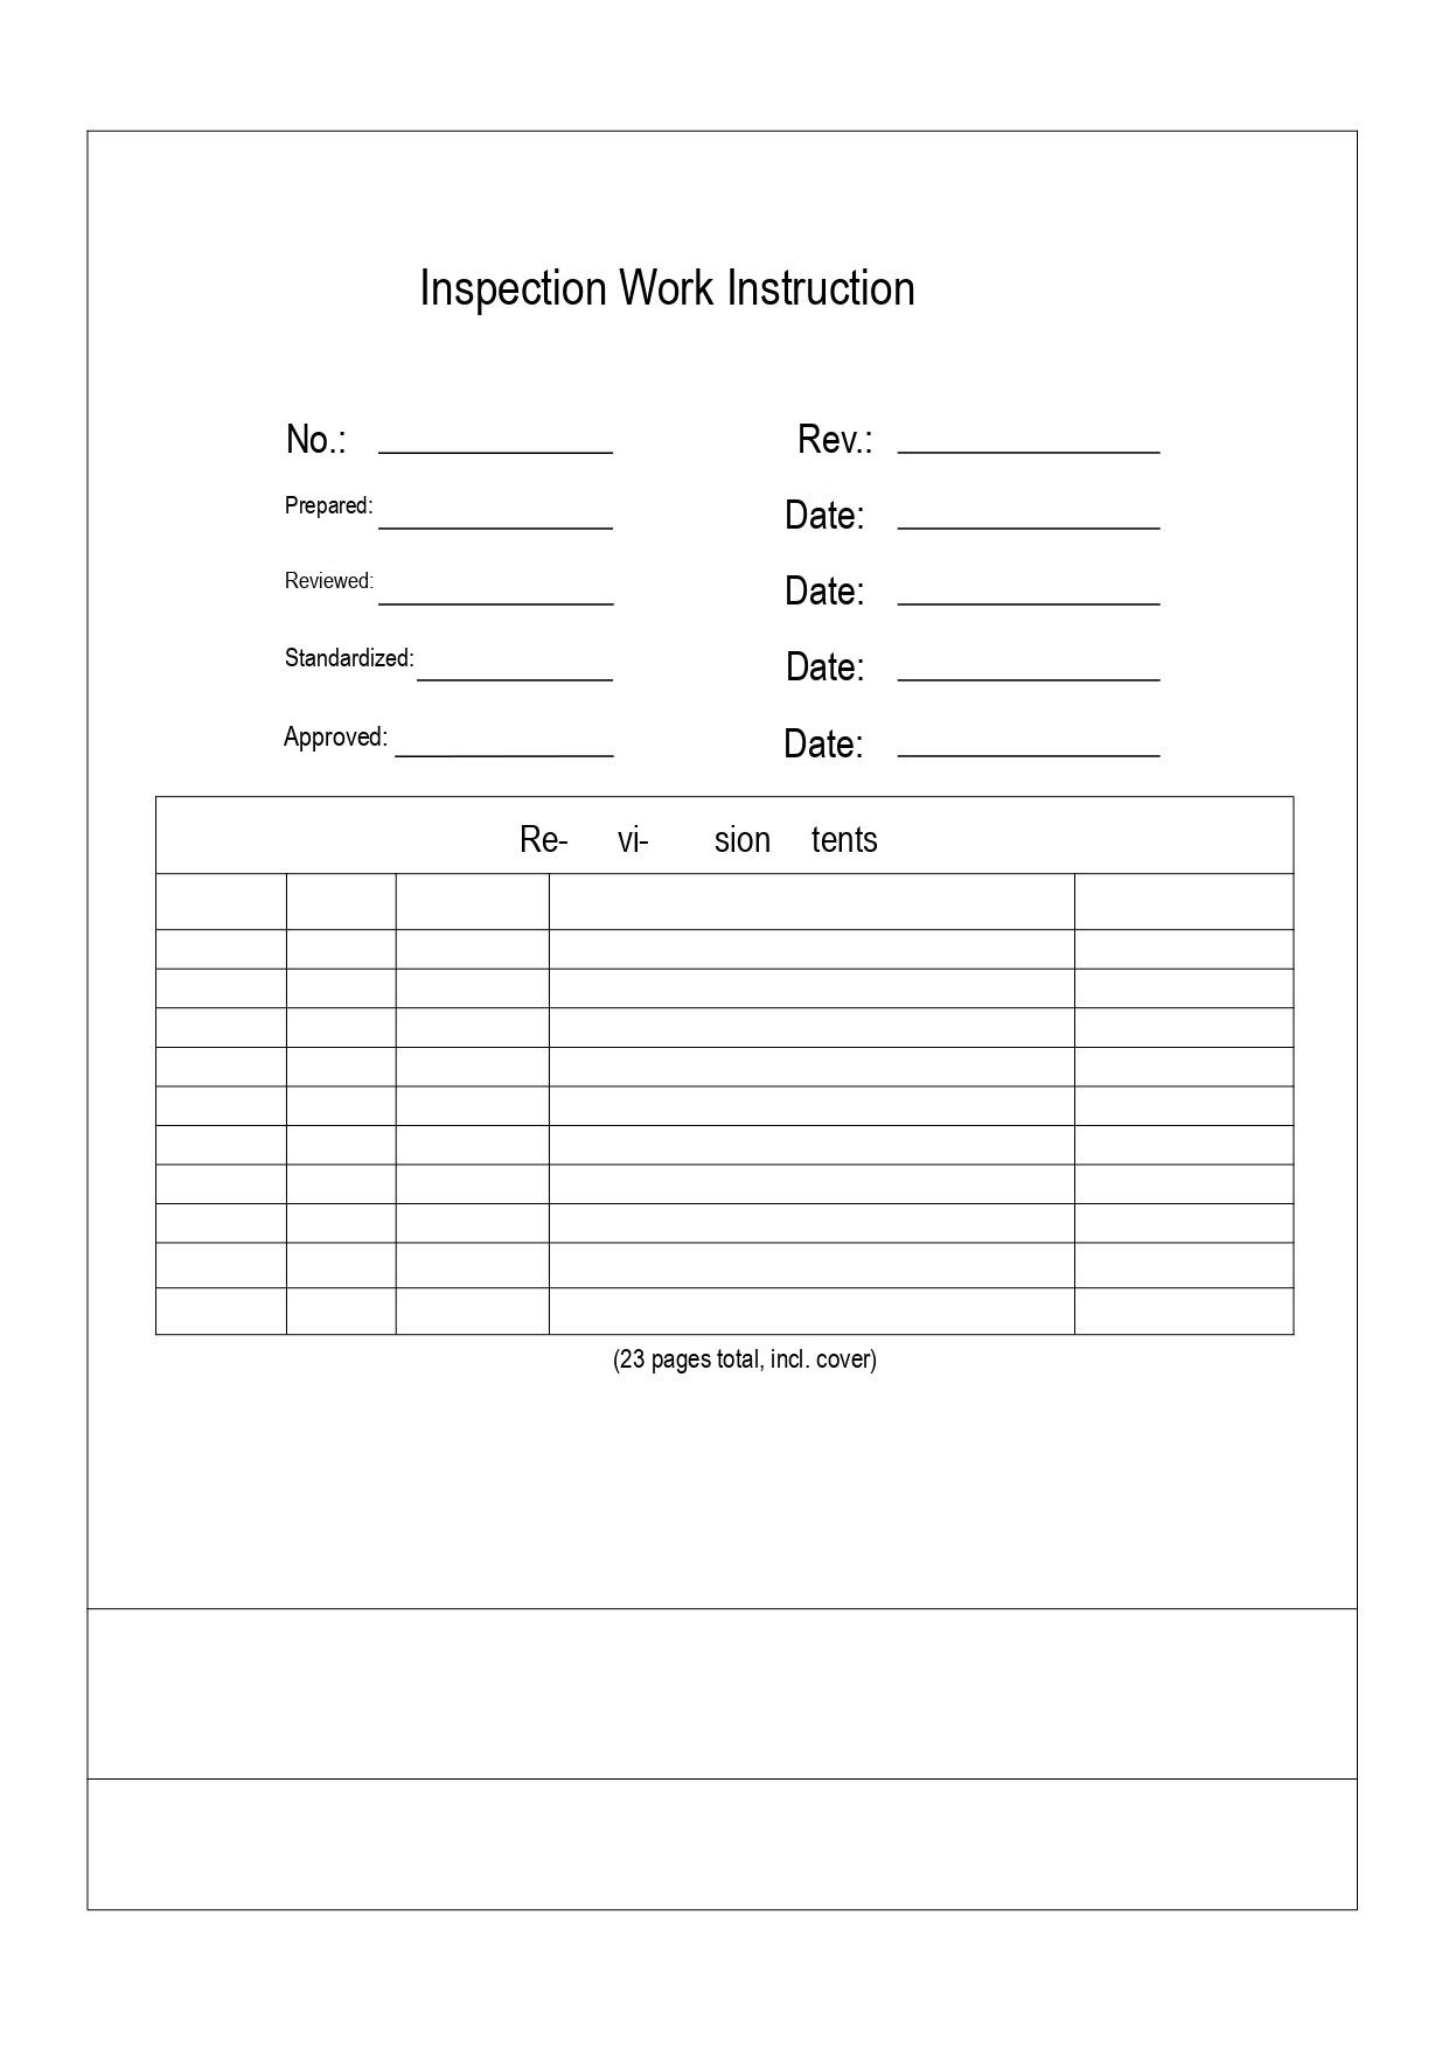Inspection Work Instruction

No.: ____________ Rev.: ____________

Prepared: ____________ Date: ____________

Reviewed: ____________ Date: ____________

Standardized: ____________ Date: ____________

Approved: ____________ Date: ____________

| Re- vi- sion tents | | | | |
|---|---|---|---|---|
| | | | | |
| | | | | |
| | | | | |
| | | | | |
| | | | | |
| | | | | |
| | | | | |
| | | | | |
| | | | | |
| | | | | |
| | | | | |

(23 pages total, incl. cover)
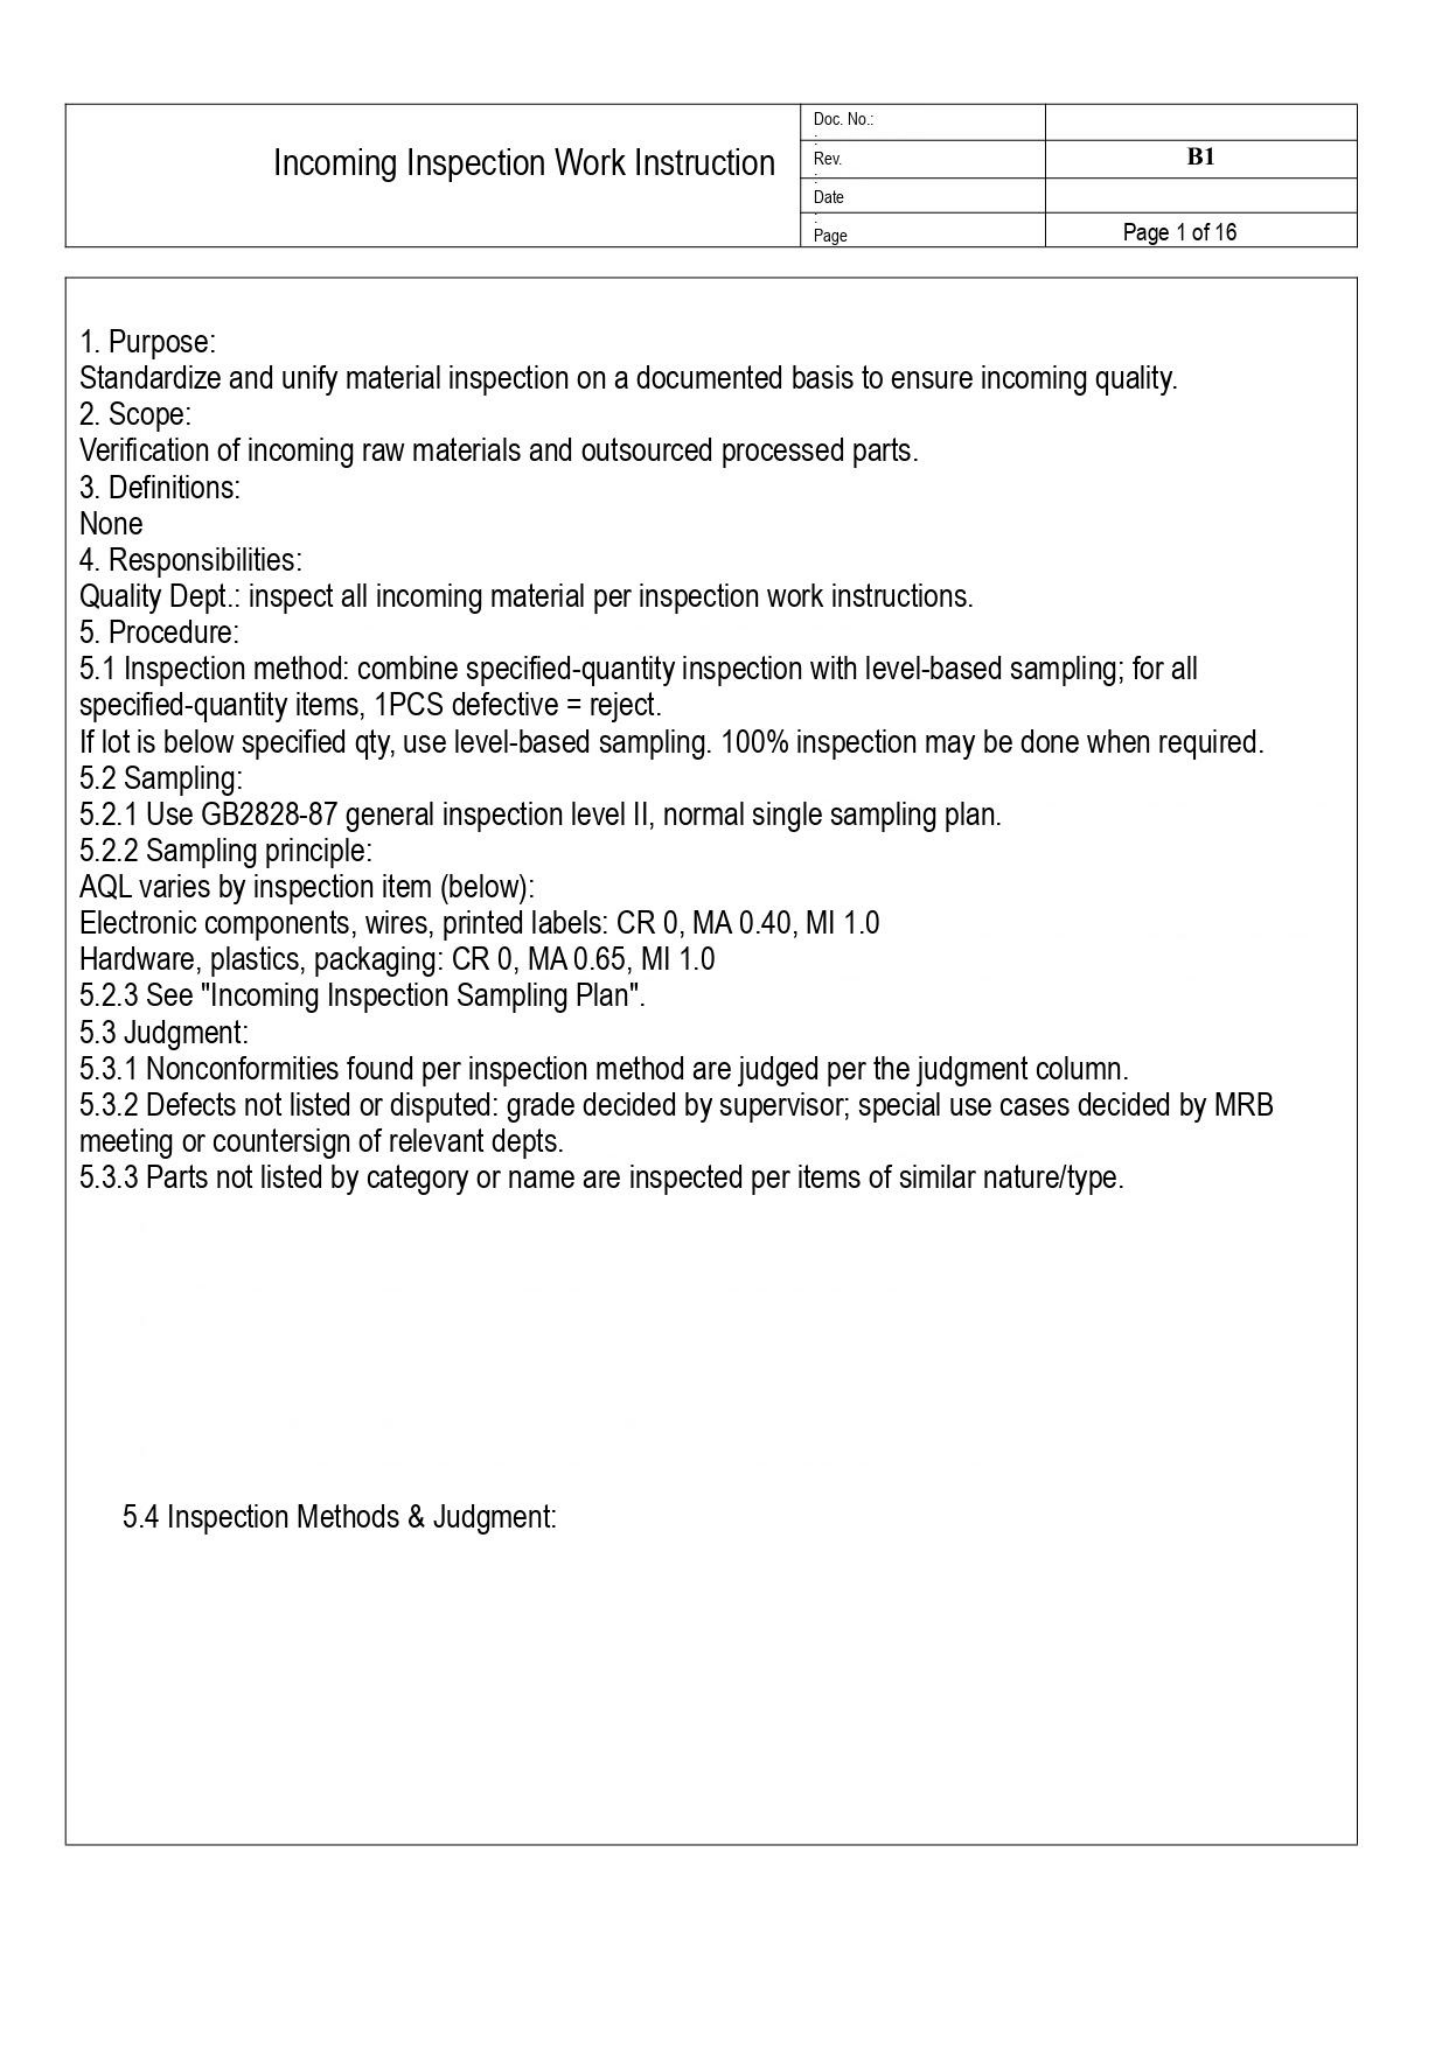Incoming Inspection Work Instruction

| Doc. No.: | |
|---|---|
| Rev. | B1 |
| Date | |
| Page | Page 1 of 16 |

1. Purpose:
Standardize and unify material inspection on a documented basis to ensure incoming quality.
2. Scope:
Verification of incoming raw materials and outsourced processed parts.
3. Definitions:
None
4. Responsibilities:
Quality Dept.: inspect all incoming material per inspection work instructions.
5. Procedure:
5.1 Inspection method: combine specified-quantity inspection with level-based sampling; for all specified-quantity items, 1PCS defective = reject.
If lot is below specified qty, use level-based sampling. 100% inspection may be done when required.
5.2 Sampling:
5.2.1 Use GB2828-87 general inspection level II, normal single sampling plan.
5.2.2 Sampling principle:
AQL varies by inspection item (below):
Electronic components, wires, printed labels: CR 0, MA 0.40, MI 1.0
Hardware, plastics, packaging: CR 0, MA 0.65, MI 1.0
5.2.3 See "Incoming Inspection Sampling Plan".
5.3 Judgment:
5.3.1 Nonconformities found per inspection method are judged per the judgment column.
5.3.2 Defects not listed or disputed: grade decided by supervisor; special use cases decided by MRB meeting or countersign of relevant depts.
5.3.3 Parts not listed by category or name are inspected per items of similar nature/type.

5.4 Inspection Methods & Judgment:
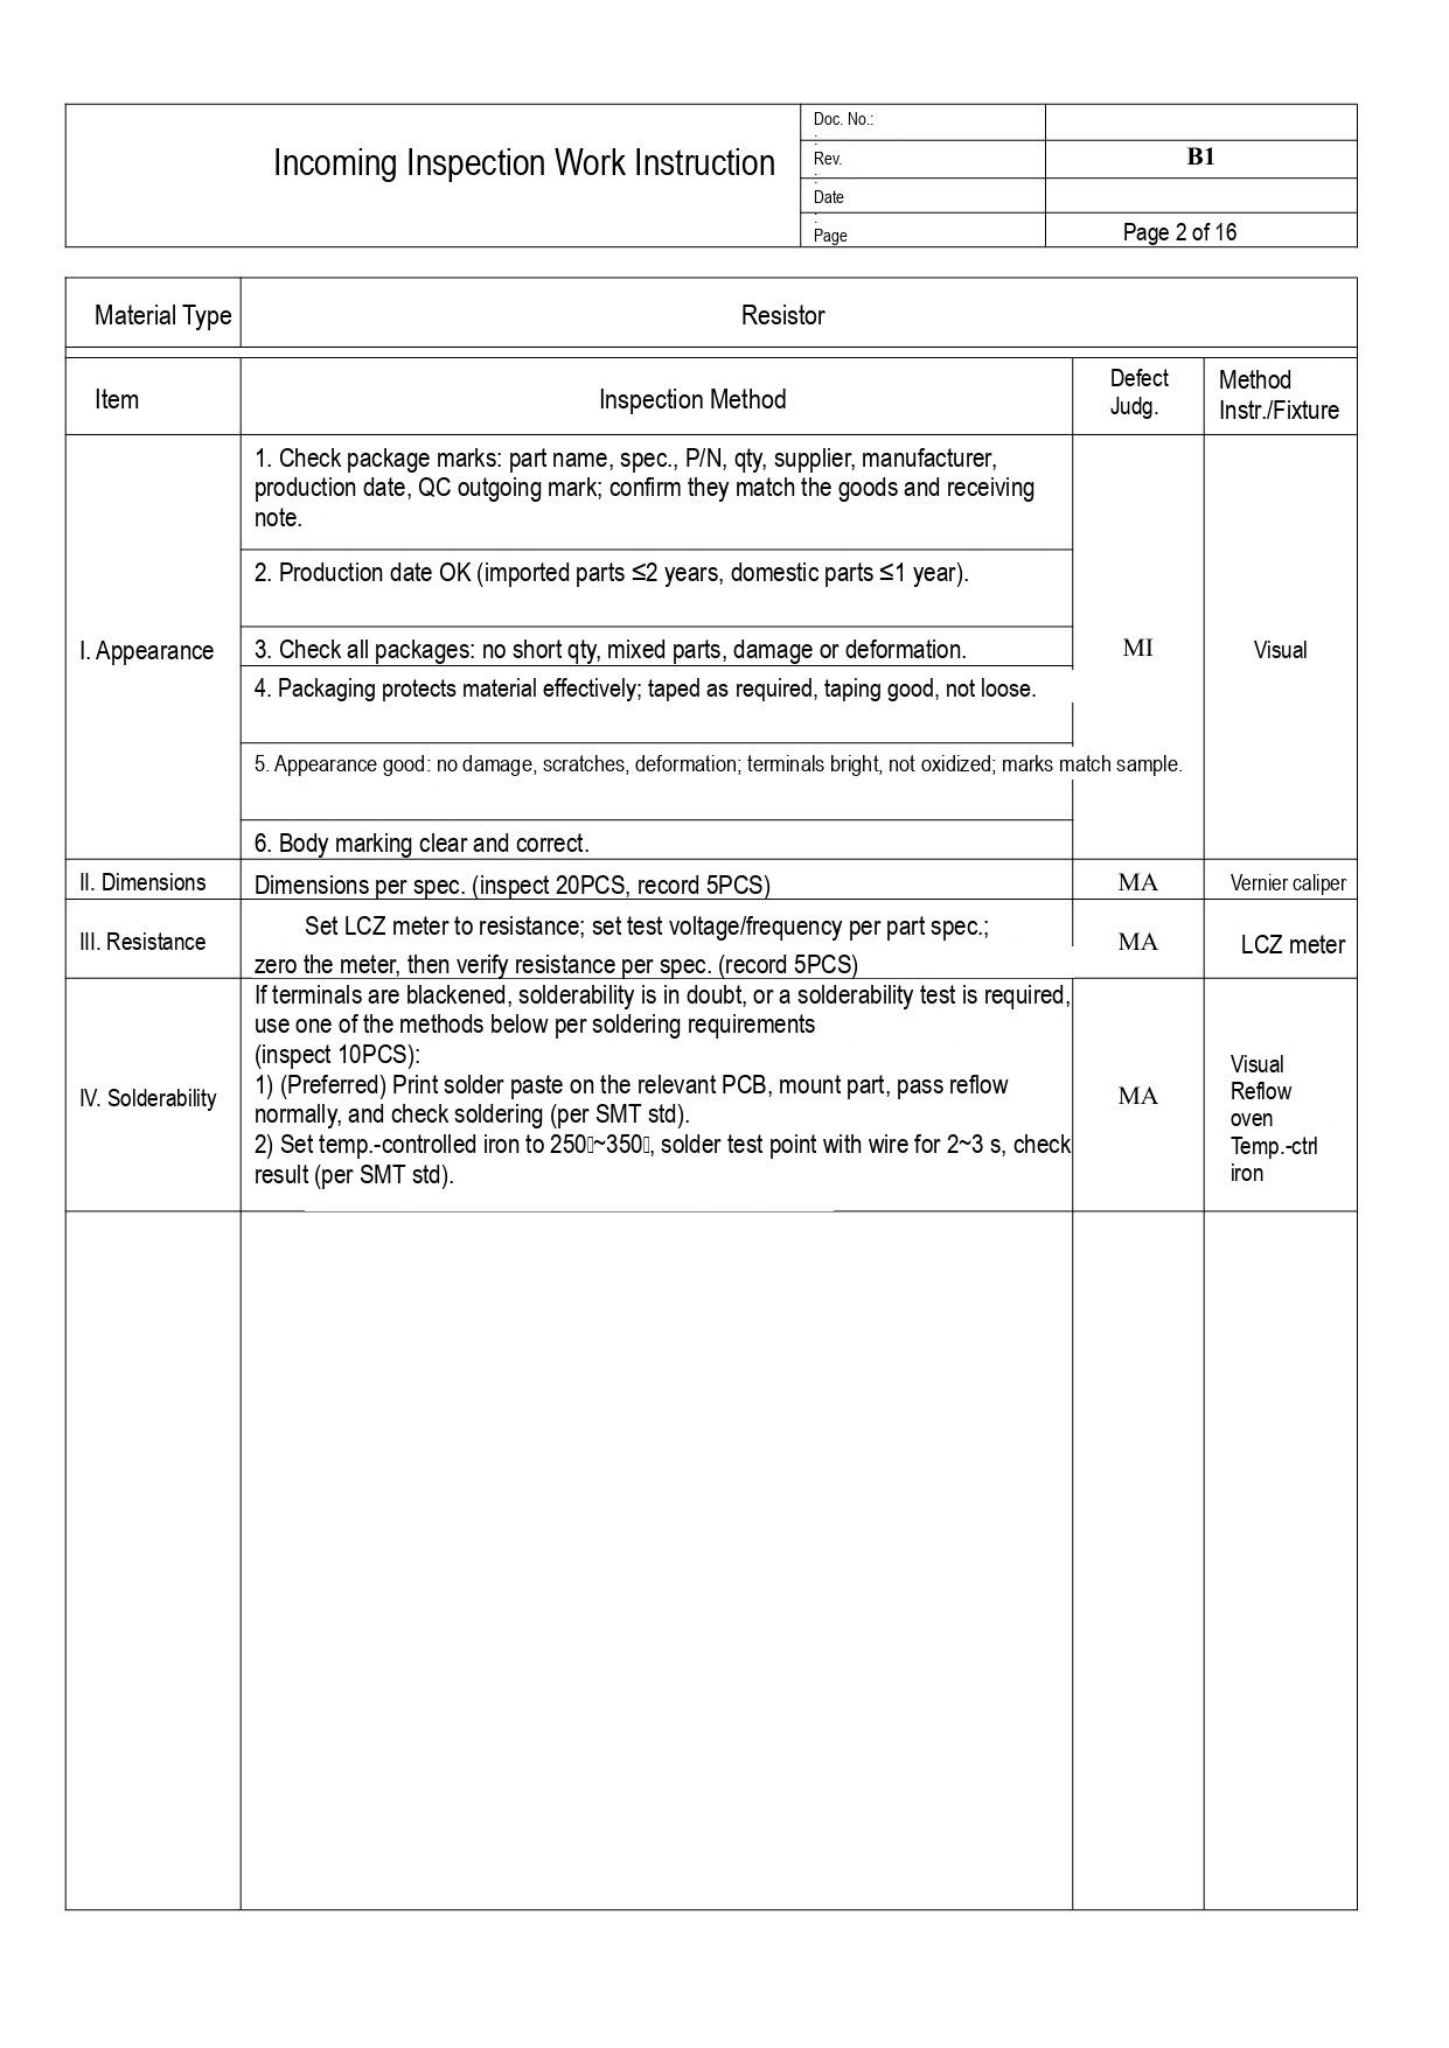Incoming Inspection Work Instruction

| Doc. No.: | |
|---|---|
| Rev. | B1 |
| Date | |
| Page | Page 2 of 16 |

| Material Type | Resistor | | |
|---|---|---|---|
| **Item** | **Inspection Method** | **Defect Judg.** | **Method Instr./Fixture** |
| I. Appearance | 1. Check package marks: part name, spec., P/N, qty, supplier, manufacturer, production date, QC outgoing mark; confirm they match the goods and receiving note.<br>2. Production date OK (imported parts ≤2 years, domestic parts ≤1 year).<br>3. Check all packages: no short qty, mixed parts, damage or deformation.<br>4. Packaging protects material effectively; taped as required, taping good, not loose.<br>5. Appearance good: no damage, scratches, deformation; terminals bright, not oxidized; marks match sample.<br>6. Body marking clear and correct. | MI | Visual |
| II. Dimensions | Dimensions per spec. (inspect 20PCS, record 5PCS) | MA | Vernier caliper |
| III. Resistance | Set LCZ meter to resistance; set test voltage/frequency per part spec.; zero the meter, then verify resistance per spec. (record 5PCS) | MA | LCZ meter |
| IV. Solderability | If terminals are blackened, solderability is in doubt, or a solderability test is required, use one of the methods below per soldering requirements (inspect 10PCS):<br>1) (Preferred) Print solder paste on the relevant PCB, mount part, pass reflow normally, and check soldering (per SMT std).<br>2) Set temp.-controlled iron to 250~350, solder test point with wire for 2~3 s, check result (per SMT std). | MA | Visual<br>Reflow oven<br>Temp.-ctrl iron |
| | | | |
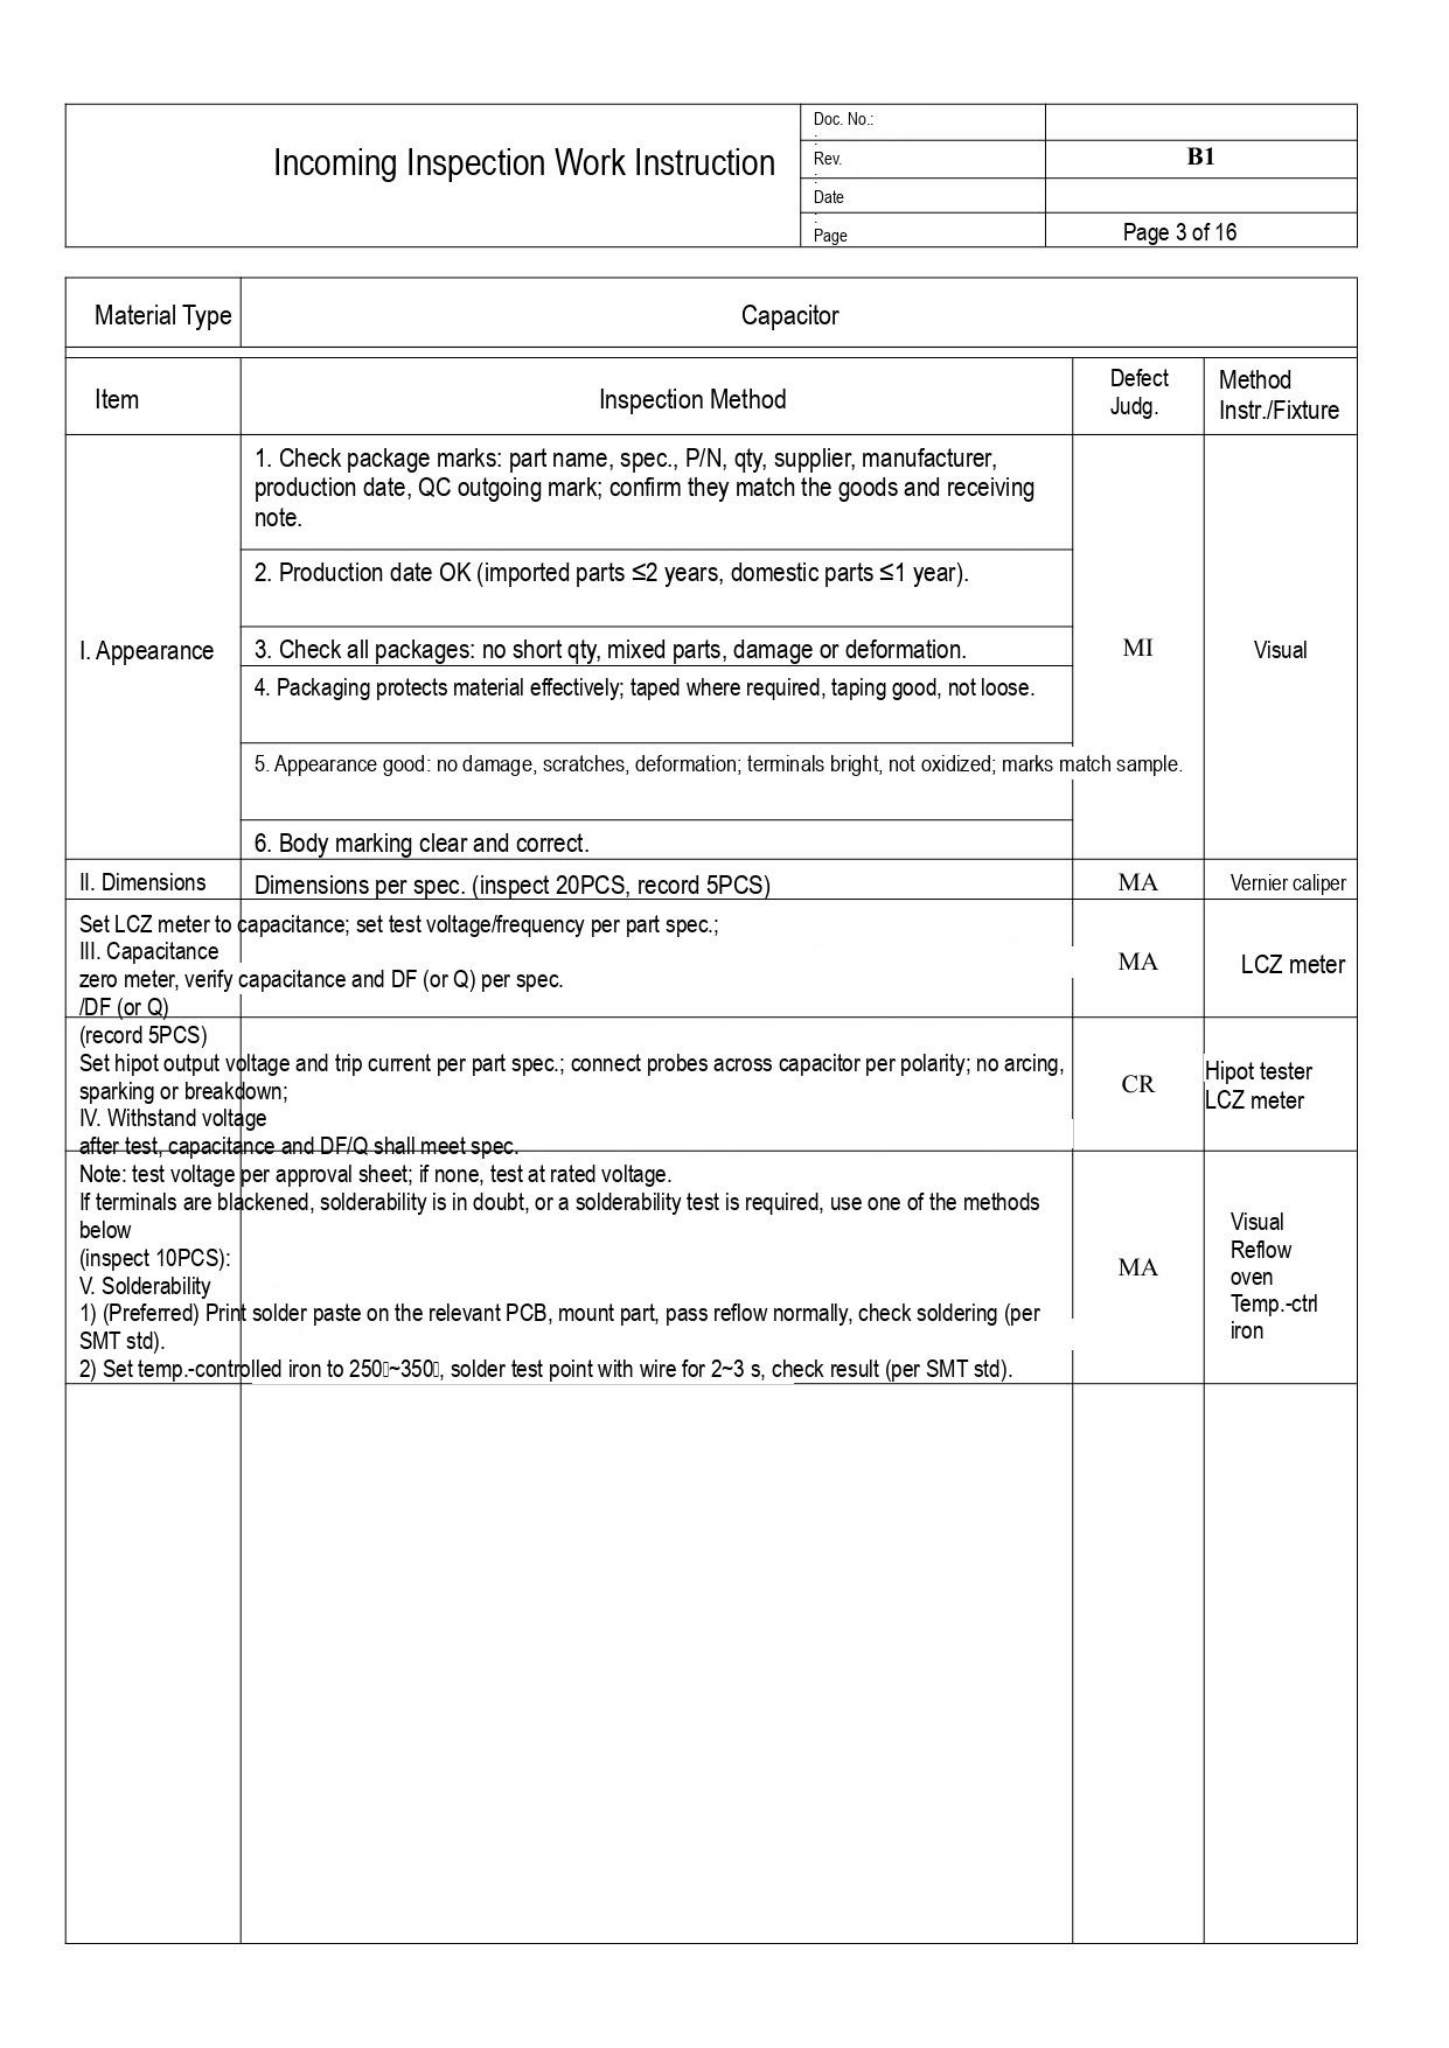# Incoming Inspection Work Instruction

| Doc. No.: | |
|---|---|
| Rev. | B1 |
| Date | |
| Page | Page 3 of 16 |

| Material Type | Capacitor |
|---|---|

| Item | Inspection Method | Defect Judg. | Method Instr./Fixture |
|---|---|---|---|
| I. Appearance | 1. Check package marks: part name, spec., P/N, qty, supplier, manufacturer, production date, QC outgoing mark; confirm they match the goods and receiving note. | MI | Visual |
| | 2. Production date OK (imported parts ≤2 years, domestic parts ≤1 year). | | |
| | 3. Check all packages: no short qty, mixed parts, damage or deformation. | | |
| | 4. Packaging protects material effectively; taped where required, taping good, not loose. | | |
| | 5. Appearance good: no damage, scratches, deformation; terminals bright, not oxidized; marks match sample. | | |
| | 6. Body marking clear and correct. | | |
| II. Dimensions | Dimensions per spec. (inspect 20PCS, record 5PCS) | MA | Vernier caliper |
| III. Capacitance /DF (or Q) | Set LCZ meter to capacitance; set test voltage/frequency per part spec.; zero meter, verify capacitance and DF (or Q) per spec. (record 5PCS) | MA | LCZ meter |
| IV. Withstand voltage | Set hipot output voltage and trip current per part spec.; connect probes across capacitor per polarity; no arcing, sparking or breakdown; after test, capacitance and DF/Q shall meet spec. | CR | Hipot tester LCZ meter |
| V. Solderability | Note: test voltage per approval sheet; if none, test at rated voltage. If terminals are blackened, solderability is in doubt, or a solderability test is required, use one of the methods below (inspect 10PCS): 1) (Preferred) Print solder paste on the relevant PCB, mount part, pass reflow normally, check soldering (per SMT std). 2) Set temp.-controlled iron to 250~350, solder test point with wire for 2~3 s, check result (per SMT std). | MA | Visual Reflow oven Temp.-ctrl iron |
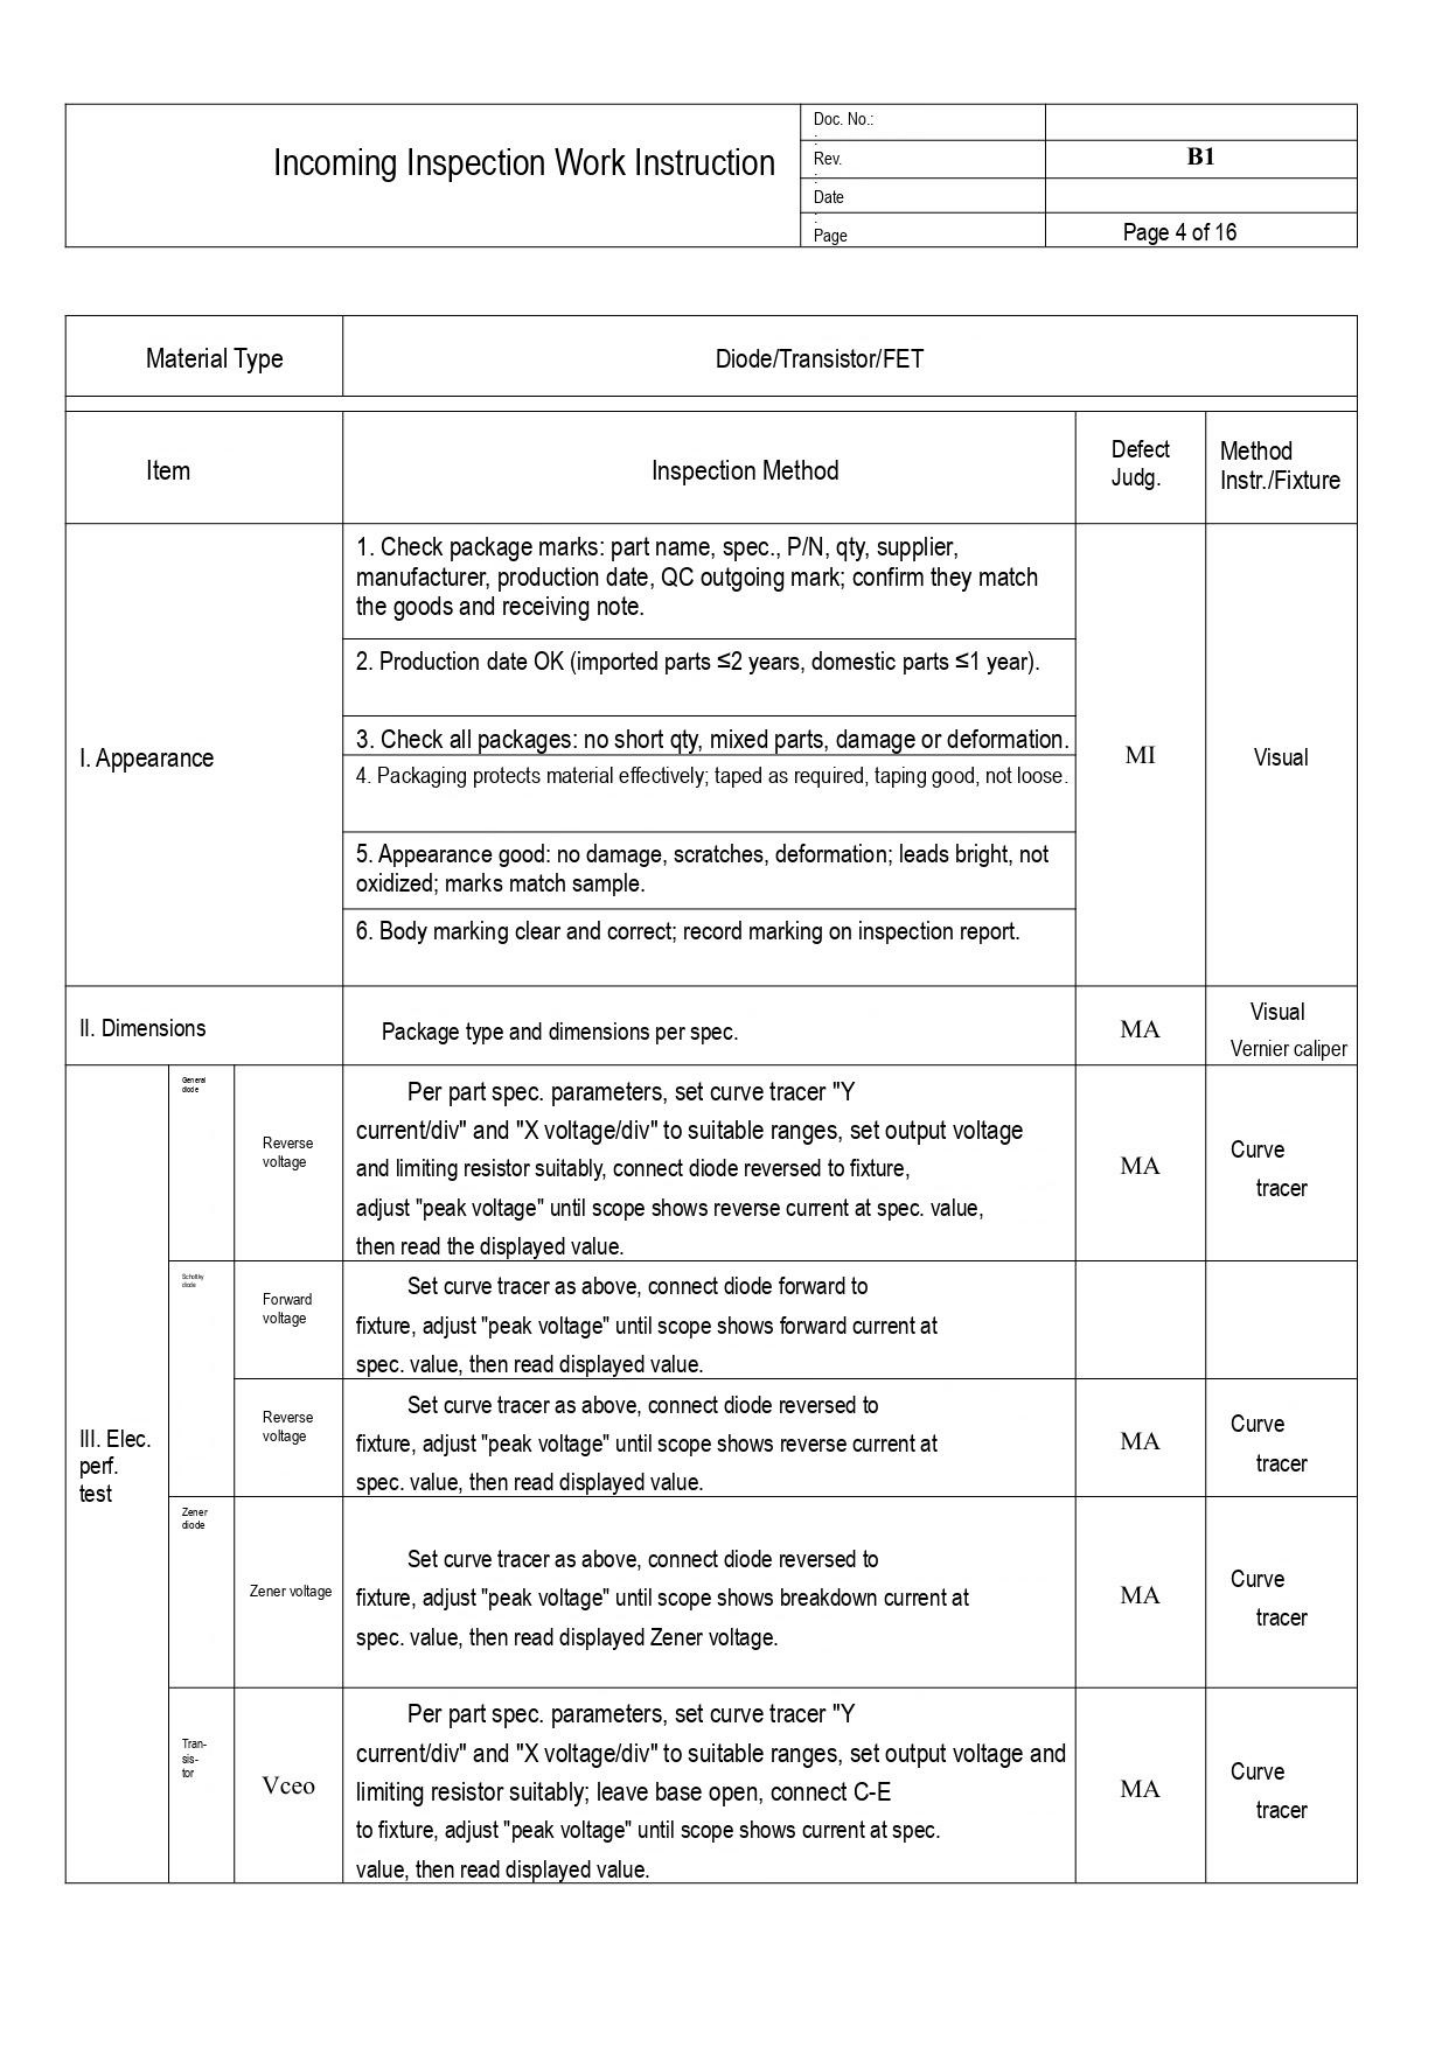Incoming Inspection Work Instruction

| Doc. No.: | |
|---|---|
| Rev. | B1 |
| Date | |
| Page | Page 4 of 16 |

| Material Type | Diode/Transistor/FET |
|---|---|

| Item | | | Inspection Method | Defect Judg. | Method Instr./Fixture |
|---|---|---|---|---|---|
| I. Appearance | | | 1. Check package marks: part name, spec., P/N, qty, supplier, manufacturer, production date, QC outgoing mark; confirm they match the goods and receiving note. | MI | Visual |
| | | | 2. Production date OK (imported parts ≤2 years, domestic parts ≤1 year). | | |
| | | | 3. Check all packages: no short qty, mixed parts, damage or deformation. | | |
| | | | 4. Packaging protects material effectively; taped as required, taping good, not loose. | | |
| | | | 5. Appearance good: no damage, scratches, deformation; leads bright, not oxidized; marks match sample. | | |
| | | | 6. Body marking clear and correct; record marking on inspection report. | | |
| II. Dimensions | | | Package type and dimensions per spec. | MA | Visual Vernier caliper |
| III. Elec. perf. test | General diode | Reverse voltage | Per part spec. parameters, set curve tracer "Y current/div" and "X voltage/div" to suitable ranges, set output voltage and limiting resistor suitably, connect diode reversed to fixture, adjust "peak voltage" until scope shows reverse current at spec. value, then read the displayed value. | MA | Curve tracer |
| | Schottky diode | Forward voltage | Set curve tracer as above, connect diode forward to fixture, adjust "peak voltage" until scope shows forward current at spec. value, then read displayed value. | | |
| | | Reverse voltage | Set curve tracer as above, connect diode reversed to fixture, adjust "peak voltage" until scope shows reverse current at spec. value, then read displayed value. | MA | Curve tracer |
| | Zener diode | Zener voltage | Set curve tracer as above, connect diode reversed to fixture, adjust "peak voltage" until scope shows breakdown current at spec. value, then read displayed Zener voltage. | MA | Curve tracer |
| | Tran-sis-tor | Vceo | Per part spec. parameters, set curve tracer "Y current/div" and "X voltage/div" to suitable ranges, set output voltage and limiting resistor suitably; leave base open, connect C-E to fixture, adjust "peak voltage" until scope shows current at spec. value, then read displayed value. | MA | Curve tracer |
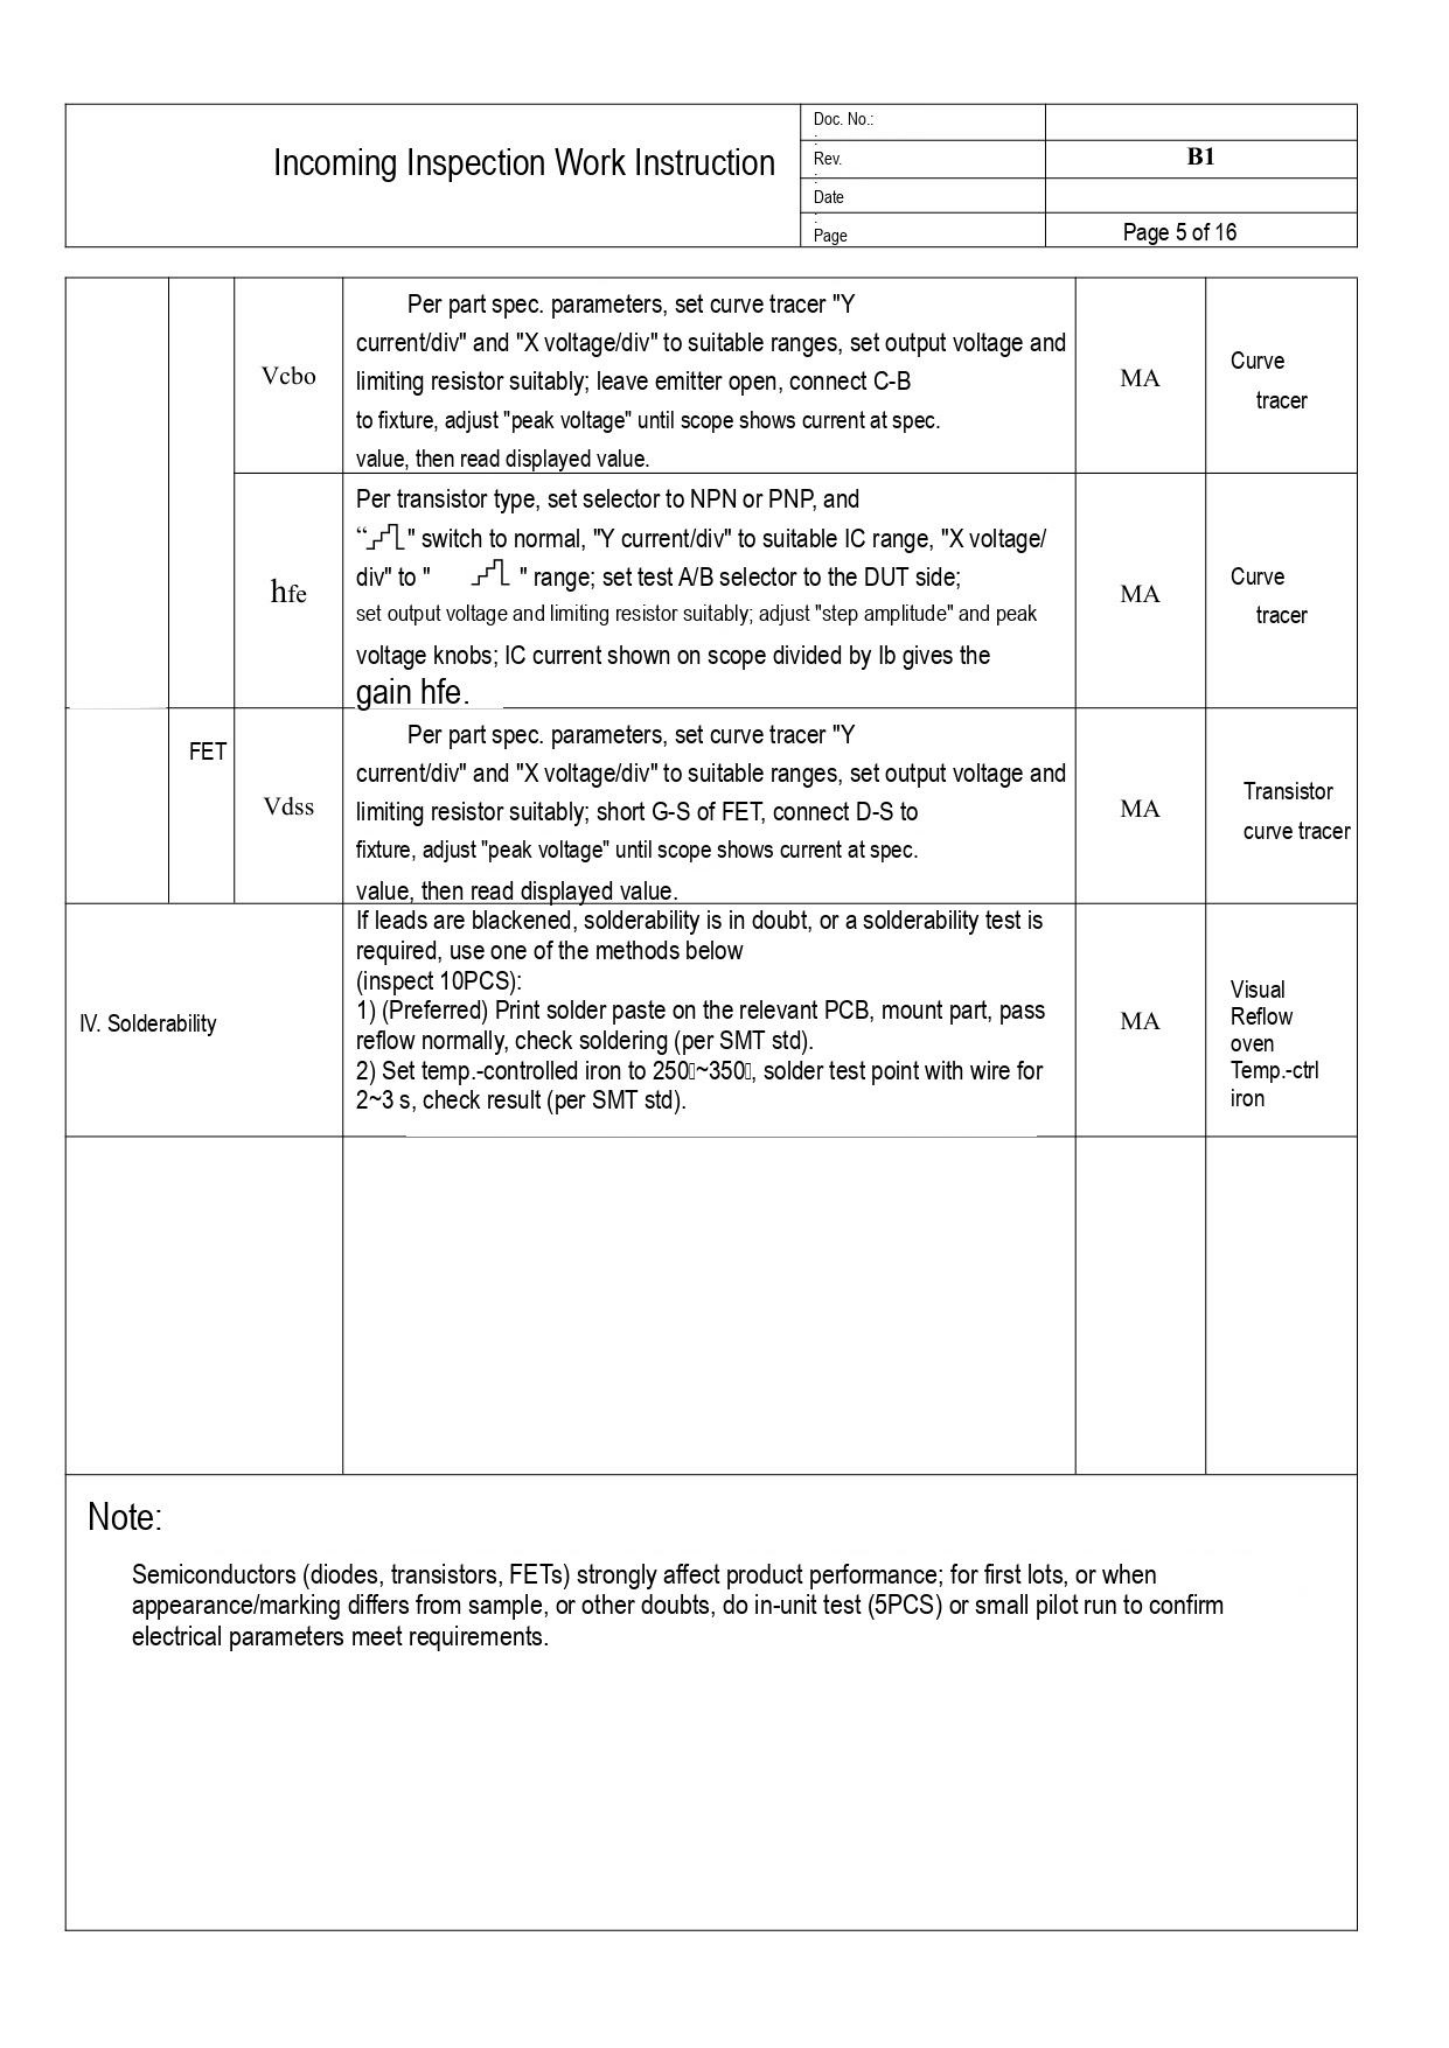| Incoming Inspection Work Instruction | Doc. No.: | |
|---|---|---|
| | Rev. | B1 |
| | Date | |
| | Page | Page 5 of 16 |

| | | | | | |
|---|---|---|---|---|---|
| | | Vcbo | Per part spec. parameters, set curve tracer "Y current/div" and "X voltage/div" to suitable ranges, set output voltage and limiting resistor suitably; leave emitter open, connect C-B to fixture, adjust "peak voltage" until scope shows current at spec. value, then read displayed value. | MA | Curve tracer |
| | | hfe | Per transistor type, set selector to NPN or PNP, and “" switch to normal, "Y current/div" to suitable IC range, "X voltage/div" to " " range; set test A/B selector to the DUT side; set output voltage and limiting resistor suitably; adjust "step amplitude" and peak voltage knobs; IC current shown on scope divided by Ib gives the gain hfe. | MA | Curve tracer |
| | FET | Vdss | Per part spec. parameters, set curve tracer "Y current/div" and "X voltage/div" to suitable ranges, set output voltage and limiting resistor suitably; short G-S of FET, connect D-S to fixture, adjust "peak voltage" until scope shows current at spec. value, then read displayed value. | MA | Transistor curve tracer |
| IV. Solderability | | | If leads are blackened, solderability is in doubt, or a solderability test is required, use one of the methods below (inspect 10PCS):<br>1) (Preferred) Print solder paste on the relevant PCB, mount part, pass reflow normally, check soldering (per SMT std).<br>2) Set temp.-controlled iron to 250□~350□, solder test point with wire for 2~3 s, check result (per SMT std). | MA | Visual<br>Reflow oven<br>Temp.-ctrl iron |
| | | | | | |

Note:

Semiconductors (diodes, transistors, FETs) strongly affect product performance; for first lots, or when appearance/marking differs from sample, or other doubts, do in-unit test (5PCS) or small pilot run to confirm electrical parameters meet requirements.
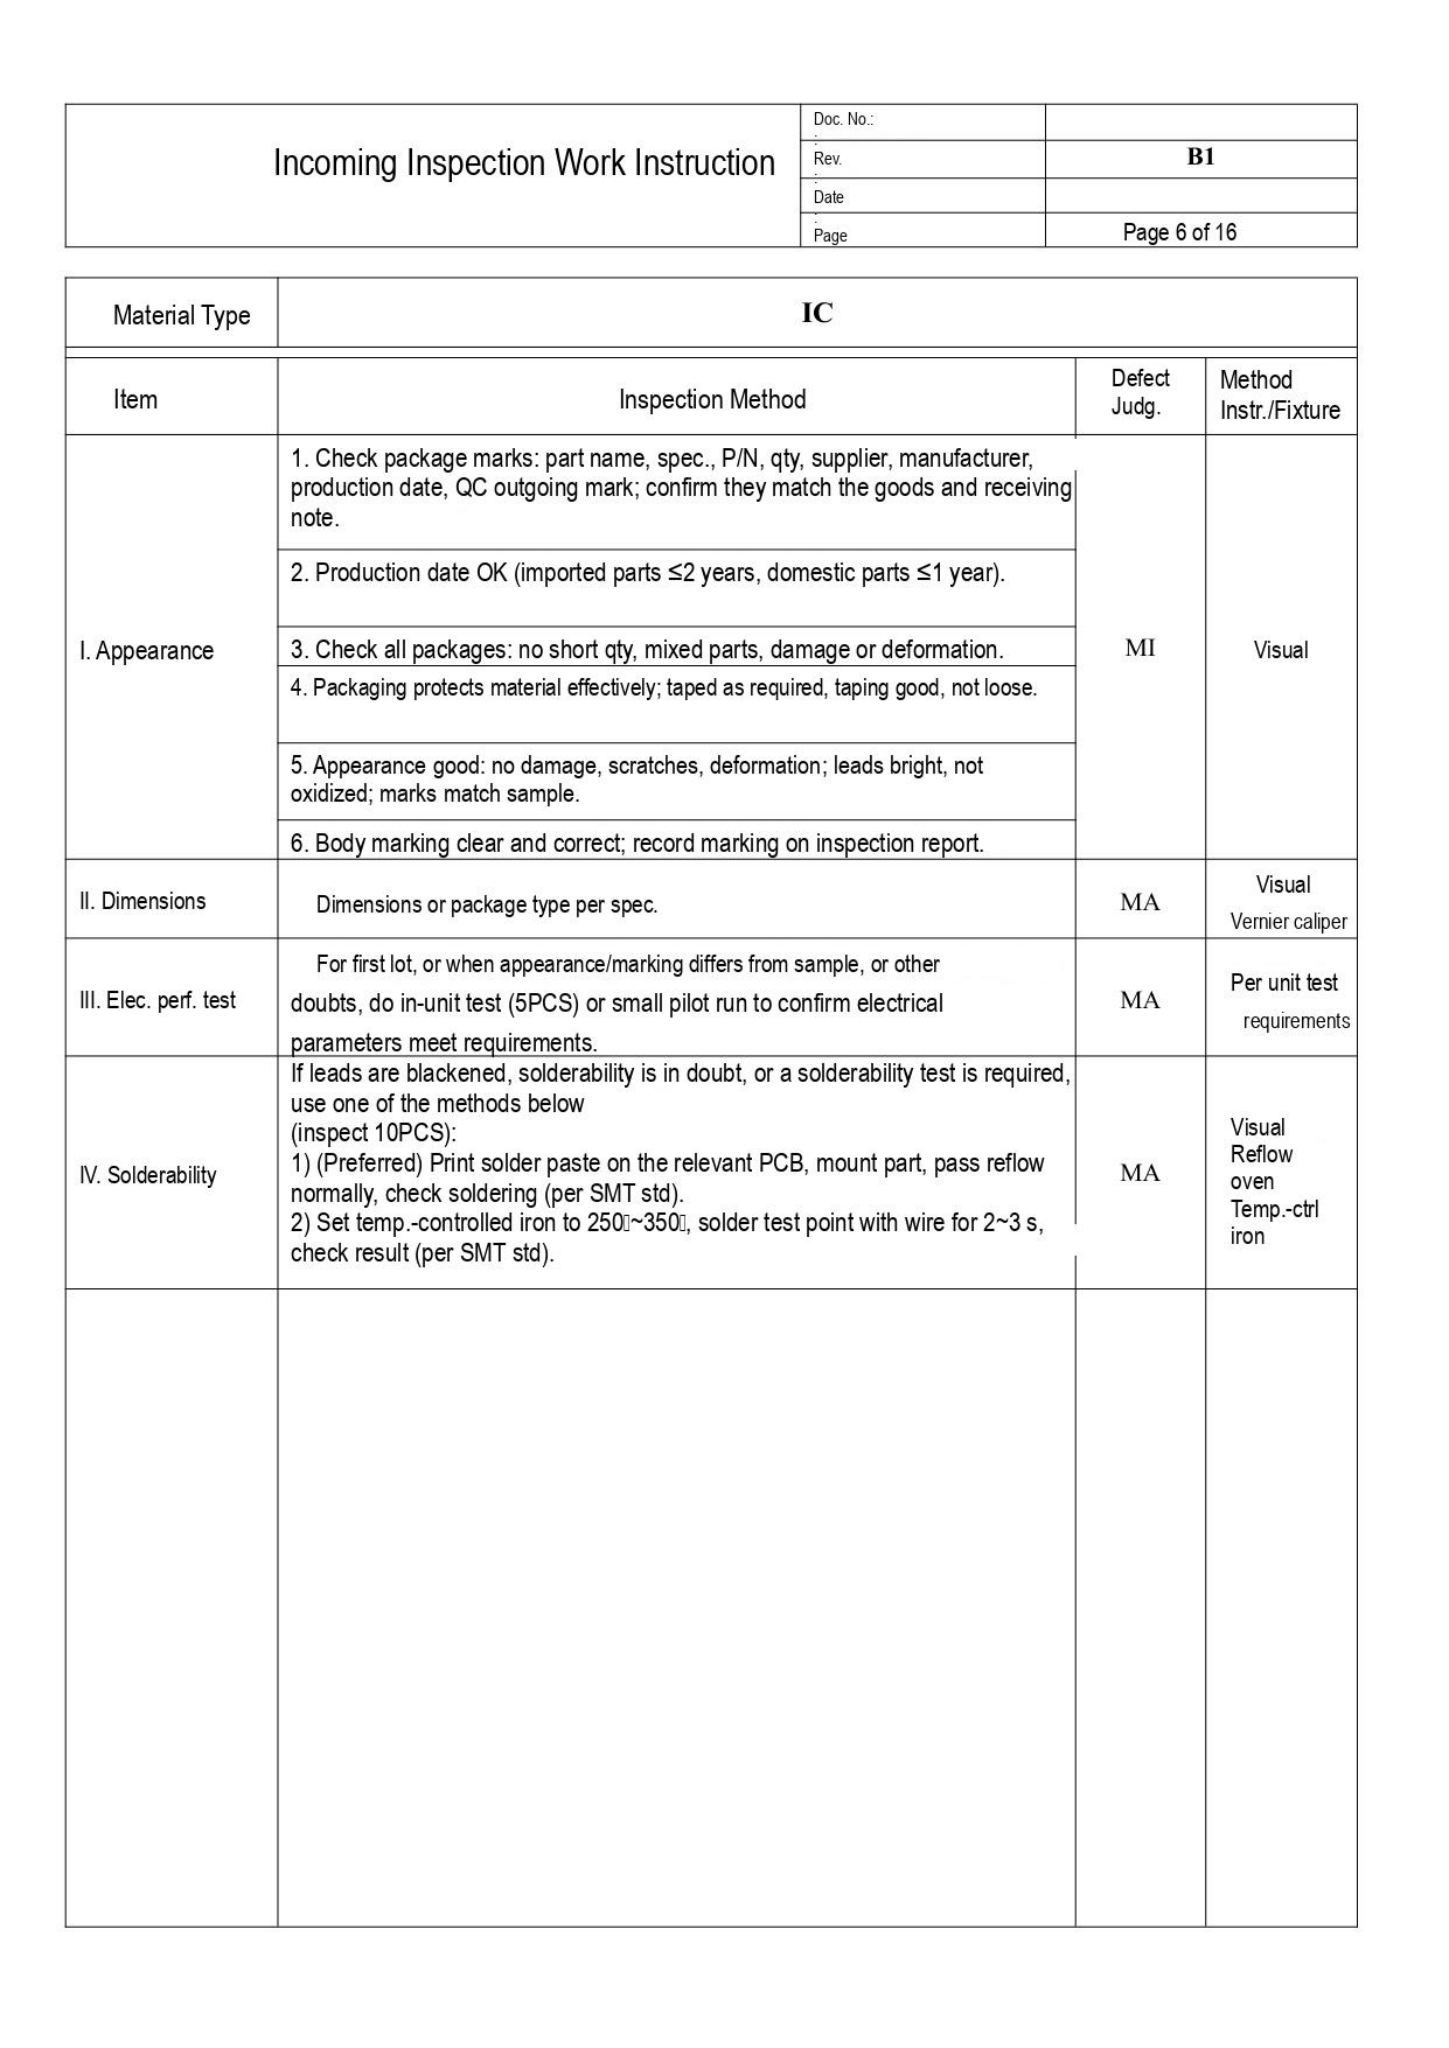# Incoming Inspection Work Instruction

| Doc. No.: | |
|---|---|
| Rev. | B1 |
| Date | |
| Page | Page 6 of 16 |

| Material Type | IC | | |
|---|---|---|---|
| **Item** | **Inspection Method** | **Defect Judg.** | **Method Instr./Fixture** |
| I. Appearance | 1. Check package marks: part name, spec., P/N, qty, supplier, manufacturer, production date, QC outgoing mark; confirm they match the goods and receiving note. | MI | Visual |
| | 2. Production date OK (imported parts ≤2 years, domestic parts ≤1 year). | | |
| | 3. Check all packages: no short qty, mixed parts, damage or deformation. | | |
| | 4. Packaging protects material effectively; taped as required, taping good, not loose. | | |
| | 5. Appearance good: no damage, scratches, deformation; leads bright, not oxidized; marks match sample. | | |
| | 6. Body marking clear and correct; record marking on inspection report. | | |
| II. Dimensions | Dimensions or package type per spec. | MA | Visual<br>Vernier caliper |
| III. Elec. perf. test | For first lot, or when appearance/marking differs from sample, or other doubts, do in-unit test (5PCS) or small pilot run to confirm electrical parameters meet requirements. | MA | Per unit test requirements |
| IV. Solderability | If leads are blackened, solderability is in doubt, or a solderability test is required, use one of the methods below<br>(inspect 10PCS):<br>1) (Preferred) Print solder paste on the relevant PCB, mount part, pass reflow normally, check soldering (per SMT std).<br>2) Set temp.-controlled iron to 250~350, solder test point with wire for 2~3 s, check result (per SMT std). | MA | Visual<br>Reflow oven<br>Temp.-ctrl iron |
| | | | |